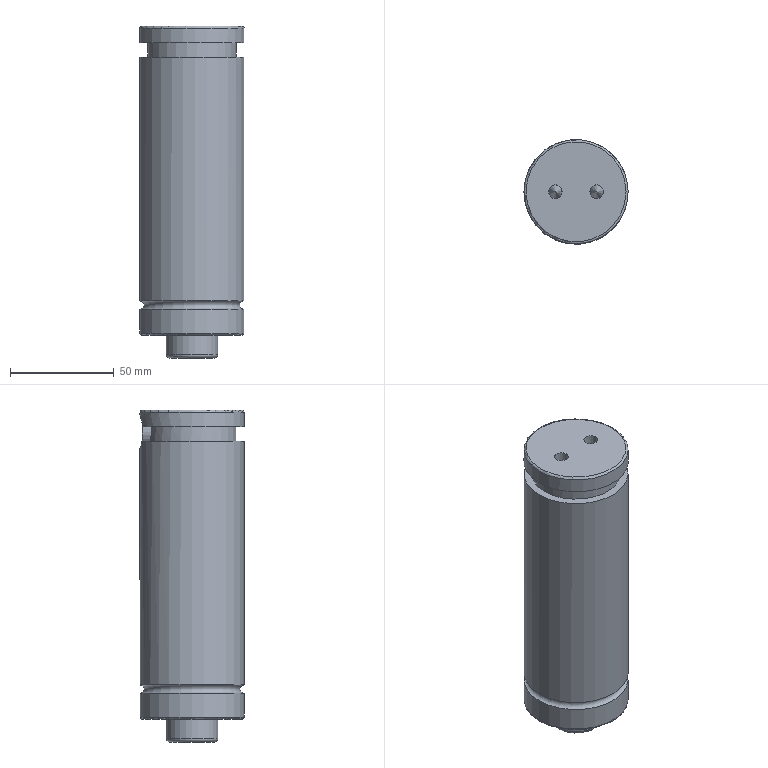Part | NX | features 1 2 | 1 solid | 38 faces | box 50.2 x 50.2 x 160 mm | volume 293536 mm3 | plane 17 | cylinder 13 | torus 4 | cone 4 | commonest cylinder face diameters 6.6 x3 14 x3 50.2 x3 10 x1 16.4 x1 25 x1
STEP:
#1=CARTESIAN_POINT('',(-260.1,5.,312.5));
#2=VERTEX_POINT('',#1);
#3=CARTESIAN_POINT('',(-235.,5.,312.5));
#4=DIRECTION('',(0.,0.,1.));
#5=DIRECTION('',(-1.,0.,0.));
#6=AXIS2_PLACEMENT_3D('',#3,#4,#5);
#7=CIRCLE('',#6,25.1);
#8=EDGE_CURVE('',#2,#2,#7,.T.);
#9=ORIENTED_EDGE('',*,*,#8,.F.);
#10=EDGE_LOOP('',(#9));
#11=FACE_BOUND('',#10,.T.);
#12=CARTESIAN_POINT('',(-260.1,5.,308.5));
#13=VERTEX_POINT('',#12);
#14=CARTESIAN_POINT('',(-235.,5.,308.5));
#15=DIRECTION('',(0.,0.,1.));
#16=DIRECTION('',(-1.,0.,0.));
#17=AXIS2_PLACEMENT_3D('',#14,#15,#16);
#18=CIRCLE('',#17,25.1);
#19=EDGE_CURVE('',#13,#13,#18,.T.);
#20=ORIENTED_EDGE('',*,*,#19,.T.);
#21=EDGE_LOOP('',(#20));
#22=FACE_BOUND('',#21,.T.);
#23=CARTESIAN_POINT('',(-235.,5.,310.5));
#24=DIRECTION('',(0.,0.,-1.));
#25=DIRECTION('',(0.,1.,0.));
#26=AXIS2_PLACEMENT_3D('',#23,#24,#25);
#27=TOROIDAL_SURFACE('',#26,25.1,2.);
#28=ADVANCED_FACE('',(#11,#22),#27,.F.);
#29=CARTESIAN_POINT('',(-260.1,5.,297.));
#30=VERTEX_POINT('',#29);
#31=CARTESIAN_POINT('',(-235.,5.,297.));
#32=DIRECTION('',(0.,0.,1.));
#33=DIRECTION('',(-1.,0.,0.));
#34=AXIS2_PLACEMENT_3D('',#31,#32,#33);
#35=CIRCLE('',#34,25.1);
#36=EDGE_CURVE('',#30,#30,#35,.T.);
#37=ORIENTED_EDGE('',*,*,#36,.F.);
#38=EDGE_LOOP('',(#37));
#39=FACE_BOUND('',#38,.T.);
#40=CARTESIAN_POINT('',(-259.1,5.,296.));
#41=VERTEX_POINT('',#40);
#42=CARTESIAN_POINT('',(-235.,5.,296.));
#43=DIRECTION('',(0.,0.,1.));
#44=DIRECTION('',(-1.,0.,0.));
#45=AXIS2_PLACEMENT_3D('',#42,#43,#44);
#46=CIRCLE('',#45,24.1);
#47=EDGE_CURVE('',#41,#41,#46,.T.);
#48=ORIENTED_EDGE('',*,*,#47,.T.);
#49=EDGE_LOOP('',(#48));
#50=FACE_BOUND('',#49,.T.);
#51=CARTESIAN_POINT('',(-235.,5.,297.));
#52=DIRECTION('',(0.,0.,-1.));
#53=DIRECTION('',(0.,1.,0.));
#54=AXIS2_PLACEMENT_3D('',#51,#52,#53);
#55=TOROIDAL_SURFACE('',#54,24.1,1.);
#56=ADVANCED_FACE('',(#39,#50),#55,.T.);
#57=ORIENTED_EDGE('',*,*,#19,.F.);
#58=EDGE_LOOP('',(#57));
#59=FACE_BOUND('',#58,.T.);
#60=ORIENTED_EDGE('',*,*,#36,.T.);
#61=EDGE_LOOP('',(#60));
#62=FACE_BOUND('',#61,.T.);
#63=CARTESIAN_POINT('',(-235.,5.,302.75));
#64=DIRECTION('',(0.,0.,1.));
#65=DIRECTION('',(0.,-1.,0.));
#66=AXIS2_PLACEMENT_3D('',#63,#64,#65);
#67=CYLINDRICAL_SURFACE('',#66,25.1);
#68=ADVANCED_FACE('',(#59,#62),#67,.T.);
#69=CARTESIAN_POINT('',(-241.855,25.167,430.));
#70=VERTEX_POINT('',#69);
#71=CARTESIAN_POINT('',(-228.145,25.167,430.));
#72=VERTEX_POINT('',#71);
#73=CARTESIAN_POINT('',(-235.,5.,430.));
#74=DIRECTION('',(0.,0.,1.));
#75=DIRECTION('',(-1.,0.,0.));
#76=AXIS2_PLACEMENT_3D('',#73,#74,#75);
#77=CIRCLE('',#76,21.3);
#78=EDGE_CURVE('',#70,#72,#77,.T.);
#79=ORIENTED_EDGE('',*,*,#78,.T.);
#80=CARTESIAN_POINT('',(-227.19,24.817,437.));
#81=VERTEX_POINT('',#80);
#82=CARTESIAN_POINT('',(-227.19,24.817,437.));
#83=CARTESIAN_POINT('',(-226.443,24.522,434.666));
#84=CARTESIAN_POINT('',(-226.814,24.714,432.028));
#85=CARTESIAN_POINT('',(-228.145,25.167,430.));
#86=B_SPLINE_CURVE_WITH_KNOTS('',3,(#82,#83,#84,#85),.UNSPECIFIED.,.F.,.F.,(4,4),(0.,0.007303),.UNSPECIFIED.);
#87=EDGE_CURVE('',#81,#72,#86,.T.);
#88=ORIENTED_EDGE('',*,*,#87,.F.);
#89=CARTESIAN_POINT('',(-242.81,24.817,437.));
#90=VERTEX_POINT('',#89);
#91=CARTESIAN_POINT('',(-235.,5.,437.));
#92=DIRECTION('',(0.,0.,1.));
#93=DIRECTION('',(-1.,0.,0.));
#94=AXIS2_PLACEMENT_3D('',#91,#92,#93);
#95=CIRCLE('',#94,21.3);
#96=EDGE_CURVE('',#90,#81,#95,.T.);
#97=ORIENTED_EDGE('',*,*,#96,.F.);
#98=CARTESIAN_POINT('',(-241.855,25.167,430.));
#99=CARTESIAN_POINT('',(-243.186,24.714,432.028));
#100=CARTESIAN_POINT('',(-243.557,24.522,434.665));
#101=CARTESIAN_POINT('',(-242.81,24.817,437.));
#102=B_SPLINE_CURVE_WITH_KNOTS('',3,(#98,#99,#100,#101),.UNSPECIFIED.,.F.,.F.,(4,4),(0.,0.007305),.UNSPECIFIED.);
#103=EDGE_CURVE('',#70,#90,#102,.T.);
#104=ORIENTED_EDGE('',*,*,#103,.F.);
#105=EDGE_LOOP('',(#79,#88,#97,#104));
#106=FACE_BOUND('',#105,.T.);
#107=CARTESIAN_POINT('',(-235.,5.,433.5));
#108=DIRECTION('',(0.,0.,1.));
#109=DIRECTION('',(0.,-1.,0.));
#110=AXIS2_PLACEMENT_3D('',#107,#108,#109);
#111=CYLINDRICAL_SURFACE('',#110,21.3);
#112=ADVANCED_FACE('',(#106),#111,.T.);
#113=CARTESIAN_POINT('',(-260.1,5.,444.));
#114=VERTEX_POINT('',#113);
#115=CARTESIAN_POINT('',(-235.,5.,444.));
#116=DIRECTION('',(0.,0.,1.));
#117=DIRECTION('',(-1.,0.,0.));
#118=AXIS2_PLACEMENT_3D('',#115,#116,#117);
#119=CIRCLE('',#118,25.1);
#120=EDGE_CURVE('',#114,#114,#119,.T.);
#121=ORIENTED_EDGE('',*,*,#120,.F.);
#122=EDGE_LOOP('',(#121));
#123=FACE_BOUND('',#122,.T.);
#124=CARTESIAN_POINT('',(-242.81,28.854,437.));
#125=VERTEX_POINT('',#124);
#126=CARTESIAN_POINT('',(-227.19,28.854,437.));
#127=VERTEX_POINT('',#126);
#128=CARTESIAN_POINT('',(-235.,5.,437.));
#129=DIRECTION('',(0.,0.,1.));
#130=DIRECTION('',(-1.,0.,0.));
#131=AXIS2_PLACEMENT_3D('',#128,#129,#130);
#132=CIRCLE('',#131,25.1);
#133=EDGE_CURVE('',#125,#127,#132,.T.);
#134=ORIENTED_EDGE('',*,*,#133,.T.);
#135=CARTESIAN_POINT('',(-242.81,28.854,437.));
#136=CARTESIAN_POINT('',(-242.278,29.028,438.662));
#137=CARTESIAN_POINT('',(-240.2,29.689,441.541));
#138=CARTESIAN_POINT('',(-234.997,30.305,443.277));
#139=CARTESIAN_POINT('',(-229.817,29.692,441.552));
#140=CARTESIAN_POINT('',(-227.722,29.028,438.661));
#141=CARTESIAN_POINT('',(-227.19,28.854,437.));
#142=B_SPLINE_CURVE_WITH_KNOTS('',3,(#135,#136,#137,#138,#139,#140,#141),.UNSPECIFIED.,.F.,.F.,(4,1,1,1,4),(-0.01037,-0.005185,-0.000001062,0.005183,0.01037),.UNSPECIFIED.);
#143=EDGE_CURVE('',#125,#127,#142,.T.);
#144=ORIENTED_EDGE('',*,*,#143,.F.);
#145=EDGE_LOOP('',(#134,#144));
#146=FACE_BOUND('',#145,.T.);
#147=CARTESIAN_POINT('',(-235.,5.,440.5));
#148=DIRECTION('',(0.,0.,1.));
#149=DIRECTION('',(0.,-1.,0.));
#150=AXIS2_PLACEMENT_3D('',#147,#148,#149);
#151=CYLINDRICAL_SURFACE('',#150,25.1);
#152=ADVANCED_FACE('',(#123,#146),#151,.T.);
#153=CARTESIAN_POINT('',(-259.1,5.,445.));
#154=VERTEX_POINT('',#153);
#155=CARTESIAN_POINT('',(-235.,5.,445.));
#156=DIRECTION('',(0.,0.,1.));
#157=DIRECTION('',(-1.,0.,0.));
#158=AXIS2_PLACEMENT_3D('',#155,#156,#157);
#159=CIRCLE('',#158,24.1);
#160=EDGE_CURVE('',#154,#154,#159,.T.);
#161=ORIENTED_EDGE('',*,*,#160,.F.);
#162=EDGE_LOOP('',(#161));
#163=FACE_BOUND('',#162,.T.);
#164=ORIENTED_EDGE('',*,*,#120,.T.);
#165=EDGE_LOOP('',(#164));
#166=FACE_BOUND('',#165,.T.);
#167=CARTESIAN_POINT('',(-235.,5.,444.));
#168=DIRECTION('',(0.,0.,-1.));
#169=DIRECTION('',(0.,1.,0.));
#170=AXIS2_PLACEMENT_3D('',#167,#168,#169);
#171=TOROIDAL_SURFACE('',#170,24.1,1.);
#172=ADVANCED_FACE('',(#163,#166),#171,.T.);
#173=CARTESIAN_POINT('',(-247.5,5.,286.5));
#174=VERTEX_POINT('',#173);
#175=CARTESIAN_POINT('',(-235.,5.,286.5));
#176=DIRECTION('',(0.,0.,1.));
#177=DIRECTION('',(-1.,0.,0.));
#178=AXIS2_PLACEMENT_3D('',#175,#176,#177);
#179=CIRCLE('',#178,12.5);
#180=EDGE_CURVE('',#174,#174,#179,.T.);
#181=ORIENTED_EDGE('',*,*,#180,.F.);
#182=EDGE_LOOP('',(#181));
#183=FACE_BOUND('',#182,.T.);
#184=CARTESIAN_POINT('',(-246.,5.,285.));
#185=VERTEX_POINT('',#184);
#186=CARTESIAN_POINT('',(-235.,5.,285.));
#187=DIRECTION('',(0.,0.,1.));
#188=DIRECTION('',(-1.,0.,0.));
#189=AXIS2_PLACEMENT_3D('',#186,#187,#188);
#190=CIRCLE('',#189,11.);
#191=EDGE_CURVE('',#185,#185,#190,.T.);
#192=ORIENTED_EDGE('',*,*,#191,.T.);
#193=EDGE_LOOP('',(#192));
#194=FACE_BOUND('',#193,.T.);
#195=CARTESIAN_POINT('',(-235.,5.,286.5));
#196=DIRECTION('',(0.,0.,-1.));
#197=DIRECTION('',(0.,1.,0.));
#198=AXIS2_PLACEMENT_3D('',#195,#196,#197);
#199=TOROIDAL_SURFACE('',#198,11.,1.5);
#200=ADVANCED_FACE('',(#183,#194),#199,.T.);
#201=CARTESIAN_POINT('',(-247.5,5.,296.));
#202=VERTEX_POINT('',#201);
#203=CARTESIAN_POINT('',(-235.,5.,296.));
#204=DIRECTION('',(0.,0.,-1.));
#205=DIRECTION('',(-1.,0.,0.));
#206=AXIS2_PLACEMENT_3D('',#203,#204,#205);
#207=CIRCLE('',#206,12.5);
#208=EDGE_CURVE('',#202,#202,#207,.T.);
#209=ORIENTED_EDGE('',*,*,#208,.T.);
#210=EDGE_LOOP('',(#209));
#211=FACE_BOUND('',#210,.T.);
#212=ORIENTED_EDGE('',*,*,#180,.T.);
#213=EDGE_LOOP('',(#212));
#214=FACE_BOUND('',#213,.T.);
#215=CARTESIAN_POINT('',(-235.,5.,291.25));
#216=DIRECTION('',(0.,0.,1.));
#217=DIRECTION('',(0.,-1.,0.));
#218=AXIS2_PLACEMENT_3D('',#215,#216,#217);
#219=CYLINDRICAL_SURFACE('',#218,12.5);
#220=ADVANCED_FACE('',(#211,#214),#219,.T.);
#221=CARTESIAN_POINT('',(-241.7,5.,432.473));
#222=VERTEX_POINT('',#221);
#223=CARTESIAN_POINT('',(-241.7,5.,436.527));
#224=VERTEX_POINT('',#223);
#225=CARTESIAN_POINT('',(-241.7,5.,434.5));
#226=DIRECTION('',(0.,0.,1.));
#227=VECTOR('',#226,1000.);
#228=LINE('',#225,#227);
#229=EDGE_CURVE('',#222,#224,#228,.T.);
#230=ORIENTED_EDGE('',*,*,#229,.F.);
#231=CARTESIAN_POINT('',(-241.7,5.,436.527));
#232=CARTESIAN_POINT('',(-241.7,5.462,436.527));
#233=CARTESIAN_POINT('',(-241.905,6.218,435.865));
#234=CARTESIAN_POINT('',(-242.047,6.453,434.502));
#235=CARTESIAN_POINT('',(-241.906,6.219,433.137));
#236=CARTESIAN_POINT('',(-241.7,5.462,432.473));
#237=CARTESIAN_POINT('',(-241.7,5.,432.473));
#238=B_SPLINE_CURVE_WITH_KNOTS('',3,(#231,#232,#233,#234,#235,#236,#237),.UNSPECIFIED.,.F.,.F.,(4,1,1,1,4),(0.,0.001359,0.002718,0.004077,0.005435),.UNSPECIFIED.);
#239=EDGE_CURVE('',#224,#222,#238,.T.);
#240=ORIENTED_EDGE('',*,*,#239,.F.);
#241=EDGE_LOOP('',(#230,#240));
#242=FACE_BOUND('',#241,.T.);
#243=CARTESIAN_POINT('',(-241.7,5.,445.));
#244=VERTEX_POINT('',#243);
#245=CARTESIAN_POINT('',(-245.,5.,445.));
#246=DIRECTION('',(0.,0.,1.));
#247=DIRECTION('',(1.,0.,0.));
#248=AXIS2_PLACEMENT_3D('',#245,#246,#247);
#249=CIRCLE('',#248,3.3);
#250=EDGE_CURVE('',#244,#244,#249,.T.);
#251=ORIENTED_EDGE('',*,*,#250,.T.);
#252=EDGE_LOOP('',(#251));
#253=FACE_BOUND('',#252,.T.);
#254=CARTESIAN_POINT('',(-241.7,5.,427.5));
#255=VERTEX_POINT('',#254);
#256=CARTESIAN_POINT('',(-245.,5.,427.5));
#257=DIRECTION('',(0.,0.,-1.));
#258=DIRECTION('',(1.,0.,0.));
#259=AXIS2_PLACEMENT_3D('',#256,#257,#258);
#260=CIRCLE('',#259,3.3);
#261=EDGE_CURVE('',#255,#255,#260,.T.);
#262=ORIENTED_EDGE('',*,*,#261,.T.);
#263=EDGE_LOOP('',(#262));
#264=FACE_BOUND('',#263,.T.);
#265=CARTESIAN_POINT('',(-245.,5.,436.25));
#266=DIRECTION('',(0.,0.,-1.));
#267=DIRECTION('',(0.,1.,0.));
#268=AXIS2_PLACEMENT_3D('',#265,#266,#267);
#269=CYLINDRICAL_SURFACE('',#268,3.3);
#270=ADVANCED_FACE('',(#242,#253,#264),#269,.F.);
#271=ORIENTED_EDGE('',*,*,#261,.F.);
#272=EDGE_LOOP('',(#271));
#273=FACE_BOUND('',#272,.T.);
#274=CARTESIAN_POINT('',(-245.,5.,436.5));
#275=VERTEX_POINT('',#274);
#276=VERTEX_LOOP('',#275);
#277=FACE_BOUND('',#276,.T.);
#278=CARTESIAN_POINT('',(-245.,5.,432.));
#279=DIRECTION('',(0.,0.,-1.));
#280=DIRECTION('',(0.,1.,0.));
#281=AXIS2_PLACEMENT_3D('',#278,#279,#280);
#282=CONICAL_SURFACE('',#281,1.65,0.3514);
#283=ADVANCED_FACE('',(#273,#277),#282,.T.);
#284=CARTESIAN_POINT('',(-225.,5.,436.5));
#285=VERTEX_POINT('',#284);
#286=VERTEX_LOOP('',#285);
#287=FACE_BOUND('',#286,.T.);
#288=CARTESIAN_POINT('',(-228.3,5.,427.5));
#289=VERTEX_POINT('',#288);
#290=CARTESIAN_POINT('',(-225.,5.,427.5));
#291=DIRECTION('',(0.,0.,1.));
#292=DIRECTION('',(-1.,0.,0.));
#293=AXIS2_PLACEMENT_3D('',#290,#291,#292);
#294=CIRCLE('',#293,3.3);
#295=EDGE_CURVE('',#289,#289,#294,.T.);
#296=ORIENTED_EDGE('',*,*,#295,.T.);
#297=EDGE_LOOP('',(#296));
#298=FACE_BOUND('',#297,.T.);
#299=CARTESIAN_POINT('',(-225.,5.,432.));
#300=DIRECTION('',(0.,0.,-1.));
#301=DIRECTION('',(0.,1.,0.));
#302=AXIS2_PLACEMENT_3D('',#299,#300,#301);
#303=CONICAL_SURFACE('',#302,1.65,0.3514);
#304=ADVANCED_FACE('',(#287,#298),#303,.T.);
#305=CARTESIAN_POINT('',(-228.3,5.,436.527));
#306=VERTEX_POINT('',#305);
#307=CARTESIAN_POINT('',(-228.3,5.,432.473));
#308=VERTEX_POINT('',#307);
#309=CARTESIAN_POINT('',(-228.3,5.,434.5));
#310=DIRECTION('',(0.,0.,-1.));
#311=VECTOR('',#310,1000.);
#312=LINE('',#309,#311);
#313=EDGE_CURVE('',#306,#308,#312,.T.);
#314=ORIENTED_EDGE('',*,*,#313,.F.);
#315=CARTESIAN_POINT('',(-228.3,5.,432.473));
#316=CARTESIAN_POINT('',(-228.3,5.462,432.473));
#317=CARTESIAN_POINT('',(-228.095,6.218,433.135));
#318=CARTESIAN_POINT('',(-227.953,6.453,434.498));
#319=CARTESIAN_POINT('',(-228.094,6.219,435.863));
#320=CARTESIAN_POINT('',(-228.3,5.462,436.527));
#321=CARTESIAN_POINT('',(-228.3,5.,436.527));
#322=B_SPLINE_CURVE_WITH_KNOTS('',3,(#315,#316,#317,#318,#319,#320,#321),.UNSPECIFIED.,.F.,.F.,(4,1,1,1,4),(0.,0.001359,0.002718,0.004077,0.005435),.UNSPECIFIED.);
#323=EDGE_CURVE('',#308,#306,#322,.T.);
#324=ORIENTED_EDGE('',*,*,#323,.F.);
#325=EDGE_LOOP('',(#314,#324));
#326=FACE_BOUND('',#325,.T.);
#327=ORIENTED_EDGE('',*,*,#295,.F.);
#328=EDGE_LOOP('',(#327));
#329=FACE_BOUND('',#328,.T.);
#330=CARTESIAN_POINT('',(-228.3,5.,445.));
#331=VERTEX_POINT('',#330);
#332=CARTESIAN_POINT('',(-225.,5.,445.));
#333=DIRECTION('',(0.,0.,1.));
#334=DIRECTION('',(-1.,0.,0.));
#335=AXIS2_PLACEMENT_3D('',#332,#333,#334);
#336=CIRCLE('',#335,3.3);
#337=EDGE_CURVE('',#331,#331,#336,.T.);
#338=ORIENTED_EDGE('',*,*,#337,.T.);
#339=EDGE_LOOP('',(#338));
#340=FACE_BOUND('',#339,.T.);
#341=CARTESIAN_POINT('',(-225.,5.,436.25));
#342=DIRECTION('',(0.,0.,1.));
#343=DIRECTION('',(0.,-1.,0.));
#344=AXIS2_PLACEMENT_3D('',#341,#342,#343);
#345=CYLINDRICAL_SURFACE('',#344,3.3);
#346=ADVANCED_FACE('',(#326,#329,#340),#345,.F.);
#347=CARTESIAN_POINT('',(-241.855,29.146,430.));
#348=VERTEX_POINT('',#347);
#349=CARTESIAN_POINT('',(-228.145,29.146,430.));
#350=VERTEX_POINT('',#349);
#351=CARTESIAN_POINT('',(-235.,5.,430.));
#352=DIRECTION('',(0.,0.,1.));
#353=DIRECTION('',(-1.,0.,0.));
#354=AXIS2_PLACEMENT_3D('',#351,#352,#353);
#355=CIRCLE('',#354,25.1);
#356=EDGE_CURVE('',#348,#350,#355,.T.);
#357=ORIENTED_EDGE('',*,*,#356,.F.);
#358=CARTESIAN_POINT('',(-228.145,29.146,430.));
#359=CARTESIAN_POINT('',(-228.891,29.358,428.863));
#360=CARTESIAN_POINT('',(-230.912,29.858,427.005));
#361=CARTESIAN_POINT('',(-235.,30.221,425.948));
#362=CARTESIAN_POINT('',(-239.087,29.858,427.004));
#363=CARTESIAN_POINT('',(-241.109,29.358,428.863));
#364=CARTESIAN_POINT('',(-241.855,29.146,430.));
#365=B_SPLINE_CURVE_WITH_KNOTS('',3,(#358,#359,#360,#361,#362,#363,#364),.UNSPECIFIED.,.F.,.F.,(4,1,1,1,4),(-0.008143,-0.004072,-0.000000126,0.004071,0.008143),.UNSPECIFIED.);
#366=EDGE_CURVE('',#350,#348,#365,.T.);
#367=ORIENTED_EDGE('',*,*,#366,.F.);
#368=EDGE_LOOP('',(#357,#367));
#369=FACE_BOUND('',#368,.T.);
#370=ORIENTED_EDGE('',*,*,#8,.T.);
#371=EDGE_LOOP('',(#370));
#372=FACE_BOUND('',#371,.T.);
#373=CARTESIAN_POINT('',(-235.,5.,371.25));
#374=DIRECTION('',(0.,0.,1.));
#375=DIRECTION('',(0.,-1.,0.));
#376=AXIS2_PLACEMENT_3D('',#373,#374,#375);
#377=CYLINDRICAL_SURFACE('',#376,25.1);
#378=ADVANCED_FACE('',(#369,#372),#377,.T.);
#379=CARTESIAN_POINT('',(-243.2,24.1,434.5));
#380=VERTEX_POINT('',#379);
#381=CARTESIAN_POINT('',(-235.,24.1,434.5));
#382=DIRECTION('',(0.,-1.,0.));
#383=DIRECTION('',(-1.,0.,0.));
#384=AXIS2_PLACEMENT_3D('',#381,#382,#383);
#385=CIRCLE('',#384,8.2);
#386=EDGE_CURVE('',#380,#380,#385,.T.);
#387=ORIENTED_EDGE('',*,*,#386,.T.);
#388=EDGE_LOOP('',(#387));
#389=FACE_BOUND('',#388,.T.);
#390=ORIENTED_EDGE('',*,*,#103,.T.);
#391=CARTESIAN_POINT('',(-242.81,27.1,437.));
#392=DIRECTION('',(0.,1.,0.));
#393=VECTOR('',#392,1000.);
#394=LINE('',#391,#393);
#395=EDGE_CURVE('',#90,#125,#394,.T.);
#396=ORIENTED_EDGE('',*,*,#395,.T.);
#397=ORIENTED_EDGE('',*,*,#143,.T.);
#398=CARTESIAN_POINT('',(-227.19,27.1,437.));
#399=DIRECTION('',(0.,-1.,0.));
#400=VECTOR('',#399,1000.);
#401=LINE('',#398,#400);
#402=EDGE_CURVE('',#127,#81,#401,.T.);
#403=ORIENTED_EDGE('',*,*,#402,.T.);
#404=ORIENTED_EDGE('',*,*,#87,.T.);
#405=CARTESIAN_POINT('',(-228.145,27.1,430.));
#406=DIRECTION('',(0.,1.,0.));
#407=VECTOR('',#406,1000.);
#408=LINE('',#405,#407);
#409=EDGE_CURVE('',#72,#350,#408,.T.);
#410=ORIENTED_EDGE('',*,*,#409,.T.);
#411=ORIENTED_EDGE('',*,*,#366,.T.);
#412=CARTESIAN_POINT('',(-241.855,27.1,430.));
#413=DIRECTION('',(0.,-1.,0.));
#414=VECTOR('',#413,1000.);
#415=LINE('',#412,#414);
#416=EDGE_CURVE('',#348,#70,#415,.T.);
#417=ORIENTED_EDGE('',*,*,#416,.T.);
#418=EDGE_LOOP('',(#390,#396,#397,#403,#404,#410,#411,#417));
#419=FACE_BOUND('',#418,.T.);
#420=CARTESIAN_POINT('',(-235.,30.1,434.5));
#421=DIRECTION('',(0.,1.,0.));
#422=DIRECTION('',(-1.,0.,0.));
#423=AXIS2_PLACEMENT_3D('',#420,#421,#422);
#424=CYLINDRICAL_SURFACE('',#423,8.2);
#425=ADVANCED_FACE('',(#389,#419),#424,.F.);
#426=CARTESIAN_POINT('',(-242.,24.1,434.5));
#427=VERTEX_POINT('',#426);
#428=CARTESIAN_POINT('',(-235.,24.1,434.5));
#429=DIRECTION('',(0.,1.,0.));
#430=DIRECTION('',(-1.,0.,0.));
#431=AXIS2_PLACEMENT_3D('',#428,#429,#430);
#432=CIRCLE('',#431,7.);
#433=EDGE_CURVE('',#427,#427,#432,.T.);
#434=ORIENTED_EDGE('',*,*,#433,.T.);
#435=EDGE_LOOP('',(#434));
#436=FACE_BOUND('',#435,.T.);
#437=CARTESIAN_POINT('',(-242.,29.1,434.5));
#438=VERTEX_POINT('',#437);
#439=CARTESIAN_POINT('',(-235.,29.1,434.5));
#440=DIRECTION('',(0.,1.,0.));
#441=DIRECTION('',(-1.,0.,0.));
#442=AXIS2_PLACEMENT_3D('',#439,#440,#441);
#443=CIRCLE('',#442,7.);
#444=EDGE_CURVE('',#438,#438,#443,.T.);
#445=ORIENTED_EDGE('',*,*,#444,.F.);
#446=EDGE_LOOP('',(#445));
#447=FACE_BOUND('',#446,.T.);
#448=CARTESIAN_POINT('',(-235.,5.,434.5));
#449=DIRECTION('',(0.,-1.,0.));
#450=DIRECTION('',(1.,0.,0.));
#451=AXIS2_PLACEMENT_3D('',#448,#449,#450);
#452=CYLINDRICAL_SURFACE('',#451,7.);
#453=ADVANCED_FACE('',(#436,#447),#452,.T.);
#454=CARTESIAN_POINT('',(-235.,5.,434.5));
#455=DIRECTION('',(0.,-1.,0.));
#456=DIRECTION('',(-1.,0.,0.));
#457=AXIS2_PLACEMENT_3D('',#454,#455,#456);
#458=CIRCLE('',#457,7.);
#459=EDGE_CURVE('',#308,#306,#458,.T.);
#460=ORIENTED_EDGE('',*,*,#459,.F.);
#461=ORIENTED_EDGE('',*,*,#323,.T.);
#462=EDGE_LOOP('',(#460,#461));
#463=FACE_BOUND('',#462,.T.);
#464=CARTESIAN_POINT('',(-235.,5.,434.5));
#465=DIRECTION('',(0.,-1.,0.));
#466=DIRECTION('',(1.,0.,0.));
#467=AXIS2_PLACEMENT_3D('',#464,#465,#466);
#468=CYLINDRICAL_SURFACE('',#467,7.);
#469=ADVANCED_FACE('',(#463),#468,.T.);
#470=ORIENTED_EDGE('',*,*,#239,.T.);
#471=CARTESIAN_POINT('',(-235.,5.,434.5));
#472=DIRECTION('',(0.,-1.,0.));
#473=DIRECTION('',(-1.,0.,0.));
#474=AXIS2_PLACEMENT_3D('',#471,#472,#473);
#475=CIRCLE('',#474,7.);
#476=EDGE_CURVE('',#224,#222,#475,.T.);
#477=ORIENTED_EDGE('',*,*,#476,.F.);
#478=EDGE_LOOP('',(#470,#477));
#479=FACE_BOUND('',#478,.T.);
#480=CARTESIAN_POINT('',(-235.,5.,434.5));
#481=DIRECTION('',(0.,-1.,0.));
#482=DIRECTION('',(1.,0.,0.));
#483=AXIS2_PLACEMENT_3D('',#480,#481,#482);
#484=CYLINDRICAL_SURFACE('',#483,7.);
#485=ADVANCED_FACE('',(#479),#484,.T.);
#486=CARTESIAN_POINT('',(-235.,-0.6,285.));
#487=VERTEX_POINT('',#486);
#488=CARTESIAN_POINT('',(-235.,5.,285.));
#489=DIRECTION('',(0.,0.,-1.));
#490=DIRECTION('',(0.,-1.,0.));
#491=AXIS2_PLACEMENT_3D('',#488,#489,#490);
#492=CIRCLE('',#491,5.6);
#493=EDGE_CURVE('',#487,#487,#492,.T.);
#494=ORIENTED_EDGE('',*,*,#493,.T.);
#495=EDGE_LOOP('',(#494));
#496=FACE_BOUND('',#495,.T.);
#497=CARTESIAN_POINT('',(-235.,0.,286.));
#498=VERTEX_POINT('',#497);
#499=CARTESIAN_POINT('',(-235.,5.,286.));
#500=DIRECTION('',(0.,0.,1.));
#501=DIRECTION('',(0.,-1.,0.));
#502=AXIS2_PLACEMENT_3D('',#499,#500,#501);
#503=CIRCLE('',#502,5.);
#504=EDGE_CURVE('',#498,#498,#503,.T.);
#505=ORIENTED_EDGE('',*,*,#504,.T.);
#506=EDGE_LOOP('',(#505));
#507=FACE_BOUND('',#506,.T.);
#508=CARTESIAN_POINT('',(-235.,5.,285.5));
#509=DIRECTION('',(0.,0.,-1.));
#510=DIRECTION('',(0.,1.,0.));
#511=AXIS2_PLACEMENT_3D('',#508,#509,#510);
#512=CONICAL_SURFACE('',#511,5.3,0.5404);
#513=ADVANCED_FACE('',(#496,#507),#512,.F.);
#514=ORIENTED_EDGE('',*,*,#504,.F.);
#515=EDGE_LOOP('',(#514));
#516=FACE_BOUND('',#515,.T.);
#517=CARTESIAN_POINT('',(-235.,0.,291.));
#518=VERTEX_POINT('',#517);
#519=CARTESIAN_POINT('',(-235.,5.,291.));
#520=DIRECTION('',(0.,0.,1.));
#521=DIRECTION('',(0.,-1.,0.));
#522=AXIS2_PLACEMENT_3D('',#519,#520,#521);
#523=CIRCLE('',#522,5.);
#524=EDGE_CURVE('',#518,#518,#523,.T.);
#525=ORIENTED_EDGE('',*,*,#524,.T.);
#526=EDGE_LOOP('',(#525));
#527=FACE_BOUND('',#526,.T.);
#528=CARTESIAN_POINT('',(-235.,5.,288.5));
#529=DIRECTION('',(0.,0.,1.));
#530=DIRECTION('',(0.,-1.,0.));
#531=AXIS2_PLACEMENT_3D('',#528,#529,#530);
#532=CYLINDRICAL_SURFACE('',#531,5.);
#533=ADVANCED_FACE('',(#516,#527),#532,.F.);
#534=CARTESIAN_POINT('',(-235.,1.7,291.));
#535=VERTEX_POINT('',#534);
#536=CARTESIAN_POINT('',(-235.,5.,291.));
#537=DIRECTION('',(0.,0.,1.));
#538=DIRECTION('',(0.,-1.,0.));
#539=AXIS2_PLACEMENT_3D('',#536,#537,#538);
#540=CIRCLE('',#539,3.3);
#541=EDGE_CURVE('',#535,#535,#540,.T.);
#542=ORIENTED_EDGE('',*,*,#541,.F.);
#543=EDGE_LOOP('',(#542));
#544=FACE_BOUND('',#543,.T.);
#545=CARTESIAN_POINT('',(-235.,1.7,299.));
#546=VERTEX_POINT('',#545);
#547=CARTESIAN_POINT('',(-235.,5.,299.));
#548=DIRECTION('',(0.,0.,1.));
#549=DIRECTION('',(0.,-1.,0.));
#550=AXIS2_PLACEMENT_3D('',#547,#548,#549);
#551=CIRCLE('',#550,3.3);
#552=EDGE_CURVE('',#546,#546,#551,.T.);
#553=ORIENTED_EDGE('',*,*,#552,.T.);
#554=EDGE_LOOP('',(#553));
#555=FACE_BOUND('',#554,.T.);
#556=CARTESIAN_POINT('',(-235.,5.,295.));
#557=DIRECTION('',(0.,0.,1.));
#558=DIRECTION('',(0.,-1.,0.));
#559=AXIS2_PLACEMENT_3D('',#556,#557,#558);
#560=CYLINDRICAL_SURFACE('',#559,3.3);
#561=ADVANCED_FACE('',(#544,#555),#560,.F.);
#562=CARTESIAN_POINT('',(-235.,5.,301.));
#563=VERTEX_POINT('',#562);
#564=VERTEX_LOOP('',#563);
#565=FACE_BOUND('',#564,.T.);
#566=ORIENTED_EDGE('',*,*,#552,.F.);
#567=EDGE_LOOP('',(#566));
#568=FACE_BOUND('',#567,.T.);
#569=CARTESIAN_POINT('',(-235.,5.,300.));
#570=DIRECTION('',(0.,0.,-1.));
#571=DIRECTION('',(0.,1.,0.));
#572=AXIS2_PLACEMENT_3D('',#569,#570,#571);
#573=CONICAL_SURFACE('',#572,1.65,1.026);
#574=ADVANCED_FACE('',(#565,#568),#573,.F.);
#575=ORIENTED_EDGE('',*,*,#524,.F.);
#576=EDGE_LOOP('',(#575));
#577=FACE_BOUND('',#576,.T.);
#578=ORIENTED_EDGE('',*,*,#541,.T.);
#579=EDGE_LOOP('',(#578));
#580=FACE_BOUND('',#579,.T.);
#581=CARTESIAN_POINT('',(-235.,0.85,291.));
#582=DIRECTION('',(0.,0.,1.));
#583=DIRECTION('',(0.,-1.,0.));
#584=AXIS2_PLACEMENT_3D('',#581,#582,#583);
#585=PLANE('',#584);
#586=ADVANCED_FACE('',(#577,#580),#585,.F.);
#587=CARTESIAN_POINT('',(-235.,29.1,431.613));
#588=VERTEX_POINT('',#587);
#589=CARTESIAN_POINT('',(-237.5,29.1,433.057));
#590=VERTEX_POINT('',#589);
#591=CARTESIAN_POINT('',(-239.148,29.1,434.008));
#592=DIRECTION('',(-0.866,0.,0.5));
#593=VECTOR('',#592,1000.);
#594=LINE('',#591,#593);
#595=EDGE_CURVE('',#588,#590,#594,.T.);
#596=ORIENTED_EDGE('',*,*,#595,.T.);
#597=CARTESIAN_POINT('',(-237.5,26.1,433.057));
#598=VERTEX_POINT('',#597);
#599=CARTESIAN_POINT('',(-237.5,30.1,433.057));
#600=DIRECTION('',(0.,-1.,0.));
#601=VECTOR('',#600,1000.);
#602=LINE('',#599,#601);
#603=EDGE_CURVE('',#590,#598,#602,.T.);
#604=ORIENTED_EDGE('',*,*,#603,.T.);
#605=CARTESIAN_POINT('',(-235.,26.1,431.613));
#606=VERTEX_POINT('',#605);
#607=CARTESIAN_POINT('',(-237.5,26.1,433.057));
#608=DIRECTION('',(0.866,0.,-0.5));
#609=VECTOR('',#608,1000.);
#610=LINE('',#607,#609);
#611=EDGE_CURVE('',#598,#606,#610,.T.);
#612=ORIENTED_EDGE('',*,*,#611,.T.);
#613=CARTESIAN_POINT('',(-235.,30.1,431.613));
#614=DIRECTION('',(0.,-1.,0.));
#615=VECTOR('',#614,1000.);
#616=LINE('',#613,#615);
#617=EDGE_CURVE('',#588,#606,#616,.T.);
#618=ORIENTED_EDGE('',*,*,#617,.F.);
#619=EDGE_LOOP('',(#596,#604,#612,#618));
#620=FACE_BOUND('',#619,.T.);
#621=CARTESIAN_POINT('',(-237.5,30.1,433.057));
#622=DIRECTION('',(-0.5,0.,-0.866));
#623=DIRECTION('',(0.866,0.,-0.5));
#624=AXIS2_PLACEMENT_3D('',#621,#622,#623);
#625=PLANE('',#624);
#626=ADVANCED_FACE('',(#620),#625,.F.);
#627=CARTESIAN_POINT('',(-237.5,29.1,435.943));
#628=VERTEX_POINT('',#627);
#629=CARTESIAN_POINT('',(-237.5,29.1,440.472));
#630=DIRECTION('',(0.,0.,1.));
#631=VECTOR('',#630,1000.);
#632=LINE('',#629,#631);
#633=EDGE_CURVE('',#590,#628,#632,.T.);
#634=ORIENTED_EDGE('',*,*,#633,.T.);
#635=CARTESIAN_POINT('',(-237.5,26.1,435.943));
#636=VERTEX_POINT('',#635);
#637=CARTESIAN_POINT('',(-237.5,30.1,435.943));
#638=DIRECTION('',(0.,-1.,0.));
#639=VECTOR('',#638,1000.);
#640=LINE('',#637,#639);
#641=EDGE_CURVE('',#628,#636,#640,.T.);
#642=ORIENTED_EDGE('',*,*,#641,.T.);
#643=CARTESIAN_POINT('',(-237.5,26.1,435.943));
#644=DIRECTION('',(0.,0.,-1.));
#645=VECTOR('',#644,1000.);
#646=LINE('',#643,#645);
#647=EDGE_CURVE('',#636,#598,#646,.T.);
#648=ORIENTED_EDGE('',*,*,#647,.T.);
#649=ORIENTED_EDGE('',*,*,#603,.F.);
#650=EDGE_LOOP('',(#634,#642,#648,#649));
#651=FACE_BOUND('',#650,.T.);
#652=CARTESIAN_POINT('',(-237.5,30.1,435.943));
#653=DIRECTION('',(-1.,0.,0.));
#654=DIRECTION('',(0.,-1.,0.));
#655=AXIS2_PLACEMENT_3D('',#652,#653,#654);
#656=PLANE('',#655);
#657=ADVANCED_FACE('',(#651),#656,.F.);
#658=CARTESIAN_POINT('',(-235.,29.1,437.387));
#659=VERTEX_POINT('',#658);
#660=CARTESIAN_POINT('',(-233.352,29.1,438.338));
#661=DIRECTION('',(0.866,0.,0.5));
#662=VECTOR('',#661,1000.);
#663=LINE('',#660,#662);
#664=EDGE_CURVE('',#628,#659,#663,.T.);
#665=ORIENTED_EDGE('',*,*,#664,.T.);
#666=CARTESIAN_POINT('',(-235.,26.1,437.387));
#667=VERTEX_POINT('',#666);
#668=CARTESIAN_POINT('',(-235.,30.1,437.387));
#669=DIRECTION('',(0.,-1.,0.));
#670=VECTOR('',#669,1000.);
#671=LINE('',#668,#670);
#672=EDGE_CURVE('',#659,#667,#671,.T.);
#673=ORIENTED_EDGE('',*,*,#672,.T.);
#674=CARTESIAN_POINT('',(-235.,26.1,437.387));
#675=DIRECTION('',(-0.866,0.,-0.5));
#676=VECTOR('',#675,1000.);
#677=LINE('',#674,#676);
#678=EDGE_CURVE('',#667,#636,#677,.T.);
#679=ORIENTED_EDGE('',*,*,#678,.T.);
#680=ORIENTED_EDGE('',*,*,#641,.F.);
#681=EDGE_LOOP('',(#665,#673,#679,#680));
#682=FACE_BOUND('',#681,.T.);
#683=CARTESIAN_POINT('',(-235.,30.1,437.387));
#684=DIRECTION('',(-0.5,0.,0.866));
#685=DIRECTION('',(-0.866,0.,-0.5));
#686=AXIS2_PLACEMENT_3D('',#683,#684,#685);
#687=PLANE('',#686);
#688=ADVANCED_FACE('',(#682),#687,.F.);
#689=CARTESIAN_POINT('',(-232.5,29.1,435.943));
#690=VERTEX_POINT('',#689);
#691=CARTESIAN_POINT('',(-235.398,29.1,437.617));
#692=DIRECTION('',(0.866,0.,-0.5));
#693=VECTOR('',#692,1000.);
#694=LINE('',#691,#693);
#695=EDGE_CURVE('',#659,#690,#694,.T.);
#696=ORIENTED_EDGE('',*,*,#695,.T.);
#697=CARTESIAN_POINT('',(-232.5,26.1,435.943));
#698=VERTEX_POINT('',#697);
#699=CARTESIAN_POINT('',(-232.5,30.1,435.943));
#700=DIRECTION('',(0.,-1.,0.));
#701=VECTOR('',#700,1000.);
#702=LINE('',#699,#701);
#703=EDGE_CURVE('',#690,#698,#702,.T.);
#704=ORIENTED_EDGE('',*,*,#703,.T.);
#705=CARTESIAN_POINT('',(-232.5,26.1,435.943));
#706=DIRECTION('',(-0.866,0.,0.5));
#707=VECTOR('',#706,1000.);
#708=LINE('',#705,#707);
#709=EDGE_CURVE('',#698,#667,#708,.T.);
#710=ORIENTED_EDGE('',*,*,#709,.T.);
#711=ORIENTED_EDGE('',*,*,#672,.F.);
#712=EDGE_LOOP('',(#696,#704,#710,#711));
#713=FACE_BOUND('',#712,.T.);
#714=CARTESIAN_POINT('',(-232.5,30.1,435.943));
#715=DIRECTION('',(0.5,0.,0.866));
#716=DIRECTION('',(-0.866,0.,0.5));
#717=AXIS2_PLACEMENT_3D('',#714,#715,#716);
#718=PLANE('',#717);
#719=ADVANCED_FACE('',(#713),#718,.F.);
#720=CARTESIAN_POINT('',(-232.5,29.1,433.057));
#721=VERTEX_POINT('',#720);
#722=CARTESIAN_POINT('',(-232.102,29.1,433.287));
#723=DIRECTION('',(-0.866,0.,-0.5));
#724=VECTOR('',#723,1000.);
#725=LINE('',#722,#724);
#726=EDGE_CURVE('',#721,#588,#725,.T.);
#727=ORIENTED_EDGE('',*,*,#726,.T.);
#728=ORIENTED_EDGE('',*,*,#617,.T.);
#729=CARTESIAN_POINT('',(-232.5,26.1,433.057));
#730=VERTEX_POINT('',#729);
#731=CARTESIAN_POINT('',(-235.,26.1,431.613));
#732=DIRECTION('',(0.866,0.,0.5));
#733=VECTOR('',#732,1000.);
#734=LINE('',#731,#733);
#735=EDGE_CURVE('',#606,#730,#734,.T.);
#736=ORIENTED_EDGE('',*,*,#735,.T.);
#737=CARTESIAN_POINT('',(-232.5,30.1,433.057));
#738=DIRECTION('',(0.,-1.,0.));
#739=VECTOR('',#738,1000.);
#740=LINE('',#737,#739);
#741=EDGE_CURVE('',#721,#730,#740,.T.);
#742=ORIENTED_EDGE('',*,*,#741,.F.);
#743=EDGE_LOOP('',(#727,#728,#736,#742));
#744=FACE_BOUND('',#743,.T.);
#745=CARTESIAN_POINT('',(-235.,30.1,431.613));
#746=DIRECTION('',(0.5,0.,-0.866));
#747=DIRECTION('',(0.866,0.,0.5));
#748=AXIS2_PLACEMENT_3D('',#745,#746,#747);
#749=PLANE('',#748);
#750=ADVANCED_FACE('',(#744),#749,.F.);
#751=CARTESIAN_POINT('',(-232.5,29.1,439.028));
#752=DIRECTION('',(0.,0.,-1.));
#753=VECTOR('',#752,1000.);
#754=LINE('',#751,#753);
#755=EDGE_CURVE('',#690,#721,#754,.T.);
#756=ORIENTED_EDGE('',*,*,#755,.T.);
#757=ORIENTED_EDGE('',*,*,#741,.T.);
#758=CARTESIAN_POINT('',(-232.5,26.1,433.057));
#759=DIRECTION('',(0.,0.,1.));
#760=VECTOR('',#759,1000.);
#761=LINE('',#758,#760);
#762=EDGE_CURVE('',#730,#698,#761,.T.);
#763=ORIENTED_EDGE('',*,*,#762,.T.);
#764=ORIENTED_EDGE('',*,*,#703,.F.);
#765=EDGE_LOOP('',(#756,#757,#763,#764));
#766=FACE_BOUND('',#765,.T.);
#767=CARTESIAN_POINT('',(-232.5,30.1,433.057));
#768=DIRECTION('',(1.,0.,0.));
#769=DIRECTION('',(0.,1.,0.));
#770=AXIS2_PLACEMENT_3D('',#767,#768,#769);
#771=PLANE('',#770);
#772=ADVANCED_FACE('',(#766),#771,.F.);
#773=ORIENTED_EDGE('',*,*,#709,.F.);
#774=ORIENTED_EDGE('',*,*,#762,.F.);
#775=ORIENTED_EDGE('',*,*,#735,.F.);
#776=ORIENTED_EDGE('',*,*,#611,.F.);
#777=ORIENTED_EDGE('',*,*,#647,.F.);
#778=ORIENTED_EDGE('',*,*,#678,.F.);
#779=EDGE_LOOP('',(#773,#774,#775,#776,#777,#778));
#780=FACE_BOUND('',#779,.T.);
#781=CARTESIAN_POINT('',(-235.,26.1,445.));
#782=DIRECTION('',(0.,1.,0.));
#783=DIRECTION('',(-1.,0.,0.));
#784=AXIS2_PLACEMENT_3D('',#781,#782,#783);
#785=PLANE('',#784);
#786=ADVANCED_FACE('',(#780),#785,.T.);
#787=ORIENTED_EDGE('',*,*,#229,.T.);
#788=ORIENTED_EDGE('',*,*,#476,.T.);
#789=EDGE_LOOP('',(#787,#788));
#790=FACE_BOUND('',#789,.T.);
#791=CARTESIAN_POINT('',(-235.,5.,445.));
#792=DIRECTION('',(0.,1.,0.));
#793=DIRECTION('',(-1.,0.,0.));
#794=AXIS2_PLACEMENT_3D('',#791,#792,#793);
#795=PLANE('',#794);
#796=ADVANCED_FACE('',(#790),#795,.F.);
#797=ORIENTED_EDGE('',*,*,#695,.F.);
#798=ORIENTED_EDGE('',*,*,#664,.F.);
#799=ORIENTED_EDGE('',*,*,#633,.F.);
#800=ORIENTED_EDGE('',*,*,#595,.F.);
#801=ORIENTED_EDGE('',*,*,#726,.F.);
#802=ORIENTED_EDGE('',*,*,#755,.F.);
#803=EDGE_LOOP('',(#797,#798,#799,#800,#801,#802));
#804=FACE_BOUND('',#803,.T.);
#805=ORIENTED_EDGE('',*,*,#444,.T.);
#806=EDGE_LOOP('',(#805));
#807=FACE_BOUND('',#806,.T.);
#808=CARTESIAN_POINT('',(-235.,29.1,445.));
#809=DIRECTION('',(0.,1.,0.));
#810=DIRECTION('',(-1.,0.,0.));
#811=AXIS2_PLACEMENT_3D('',#808,#809,#810);
#812=PLANE('',#811);
#813=ADVANCED_FACE('',(#804,#807),#812,.T.);
#814=ORIENTED_EDGE('',*,*,#313,.T.);
#815=ORIENTED_EDGE('',*,*,#459,.T.);
#816=EDGE_LOOP('',(#814,#815));
#817=FACE_BOUND('',#816,.T.);
#818=CARTESIAN_POINT('',(-235.,5.,445.));
#819=DIRECTION('',(0.,1.,0.));
#820=DIRECTION('',(-1.,0.,0.));
#821=AXIS2_PLACEMENT_3D('',#818,#819,#820);
#822=PLANE('',#821);
#823=ADVANCED_FACE('',(#817),#822,.F.);
#824=ORIENTED_EDGE('',*,*,#433,.F.);
#825=EDGE_LOOP('',(#824));
#826=FACE_BOUND('',#825,.T.);
#827=ORIENTED_EDGE('',*,*,#386,.F.);
#828=EDGE_LOOP('',(#827));
#829=FACE_BOUND('',#828,.T.);
#830=CARTESIAN_POINT('',(-235.,24.1,445.));
#831=DIRECTION('',(0.,1.,0.));
#832=DIRECTION('',(-1.,0.,0.));
#833=AXIS2_PLACEMENT_3D('',#830,#831,#832);
#834=PLANE('',#833);
#835=ADVANCED_FACE('',(#826,#829),#834,.T.);
#836=ORIENTED_EDGE('',*,*,#493,.F.);
#837=EDGE_LOOP('',(#836));
#838=FACE_BOUND('',#837,.T.);
#839=ORIENTED_EDGE('',*,*,#191,.F.);
#840=EDGE_LOOP('',(#839));
#841=FACE_BOUND('',#840,.T.);
#842=CARTESIAN_POINT('',(-240.5,5.,285.));
#843=DIRECTION('',(0.,0.,-1.));
#844=DIRECTION('',(0.,1.,0.));
#845=AXIS2_PLACEMENT_3D('',#842,#843,#844);
#846=PLANE('',#845);
#847=ADVANCED_FACE('',(#838,#841),#846,.T.);
#848=ORIENTED_EDGE('',*,*,#337,.F.);
#849=EDGE_LOOP('',(#848));
#850=FACE_BOUND('',#849,.T.);
#851=ORIENTED_EDGE('',*,*,#250,.F.);
#852=EDGE_LOOP('',(#851));
#853=FACE_BOUND('',#852,.T.);
#854=ORIENTED_EDGE('',*,*,#160,.T.);
#855=EDGE_LOOP('',(#854));
#856=FACE_BOUND('',#855,.T.);
#857=CARTESIAN_POINT('',(-247.05,5.,445.));
#858=DIRECTION('',(0.,0.,1.));
#859=DIRECTION('',(-1.,0.,0.));
#860=AXIS2_PLACEMENT_3D('',#857,#858,#859);
#861=PLANE('',#860);
#862=ADVANCED_FACE('',(#850,#853,#856),#861,.T.);
#863=ORIENTED_EDGE('',*,*,#402,.F.);
#864=ORIENTED_EDGE('',*,*,#133,.F.);
#865=ORIENTED_EDGE('',*,*,#395,.F.);
#866=ORIENTED_EDGE('',*,*,#96,.T.);
#867=EDGE_LOOP('',(#863,#864,#865,#866));
#868=FACE_BOUND('',#867,.T.);
#869=CARTESIAN_POINT('',(-258.2,5.,437.));
#870=DIRECTION('',(0.,0.,-1.));
#871=DIRECTION('',(0.,1.,0.));
#872=AXIS2_PLACEMENT_3D('',#869,#870,#871);
#873=PLANE('',#872);
#874=ADVANCED_FACE('',(#868),#873,.T.);
#875=ORIENTED_EDGE('',*,*,#409,.F.);
#876=ORIENTED_EDGE('',*,*,#78,.F.);
#877=ORIENTED_EDGE('',*,*,#416,.F.);
#878=ORIENTED_EDGE('',*,*,#356,.T.);
#879=EDGE_LOOP('',(#875,#876,#877,#878));
#880=FACE_BOUND('',#879,.T.);
#881=CARTESIAN_POINT('',(-258.2,5.,430.));
#882=DIRECTION('',(0.,0.,1.));
#883=DIRECTION('',(0.,-1.,0.));
#884=AXIS2_PLACEMENT_3D('',#881,#882,#883);
#885=PLANE('',#884);
#886=ADVANCED_FACE('',(#880),#885,.T.);
#887=ORIENTED_EDGE('',*,*,#208,.F.);
#888=EDGE_LOOP('',(#887));
#889=FACE_BOUND('',#888,.T.);
#890=ORIENTED_EDGE('',*,*,#47,.F.);
#891=EDGE_LOOP('',(#890));
#892=FACE_BOUND('',#891,.T.);
#893=CARTESIAN_POINT('',(-247.05,5.,296.));
#894=DIRECTION('',(0.,0.,-1.));
#895=DIRECTION('',(0.,1.,0.));
#896=AXIS2_PLACEMENT_3D('',#893,#894,#895);
#897=PLANE('',#896);
#898=ADVANCED_FACE('',(#889,#892),#897,.T.);
#899=CLOSED_SHELL('',(#28,#56,#68,#112,#152,#172,#200,#220,#270,#283,#304,#346,#378,#425,#453,#469,#485,#513,#533,#561,#574,#586,#626,#657,#688,#719,#750,#772,#786,#796,#813,#823,#835,#847,#862,#874,#886,#898));
#900=MANIFOLD_SOLID_BREP('',#899);
#901=(LENGTH_UNIT()NAMED_UNIT(*)SI_UNIT(.MILLI.,.METRE.));
#902=UNCERTAINTY_MEASURE_WITH_UNIT(LENGTH_MEASURE(0.0508),#901,'','');
#903=(NAMED_UNIT(*)PLANE_ANGLE_UNIT()SI_UNIT($,.RADIAN.));
#904=(NAMED_UNIT(*)SI_UNIT($,.STERADIAN.)SOLID_ANGLE_UNIT());
#905=(GEOMETRIC_REPRESENTATION_CONTEXT(3)GLOBAL_UNCERTAINTY_ASSIGNED_CONTEXT((#902))GLOBAL_UNIT_ASSIGNED_CONTEXT((#901,#903,#904))REPRESENTATION_CONTEXT('',''));
#906=ADVANCED_BREP_SHAPE_REPRESENTATION('',(#900),#905);